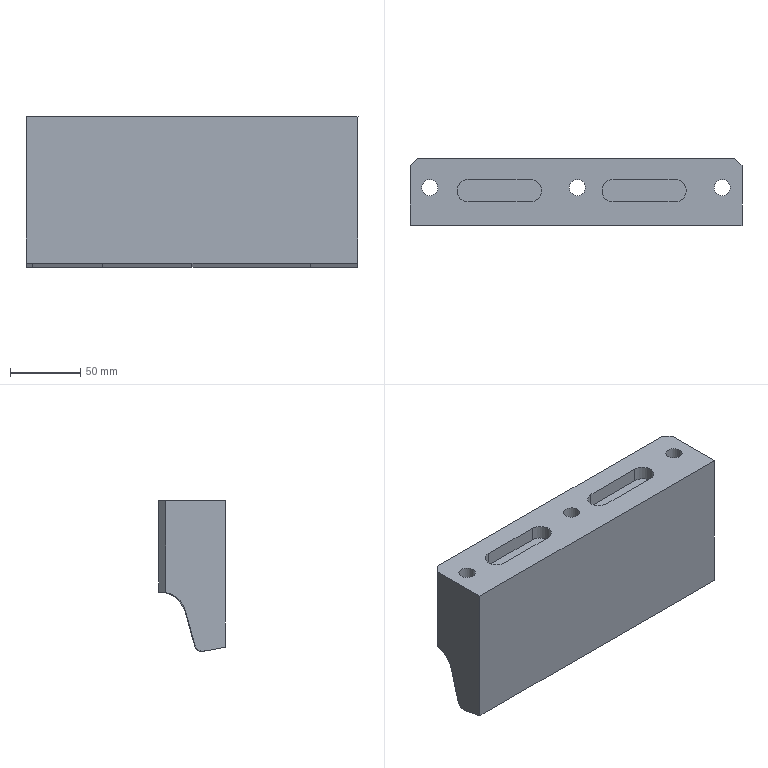Part | NX | features solid 2 | 1 solid | 46 faces | box 236 x 47.451 x 107.196 mm | volume 916889 mm3 | plane 17 | spline 15 | cylinder 12 | cone 2 | commonest cylinder face diameters 16 x4 11.507 x3 18.008 x3 8.506 x2